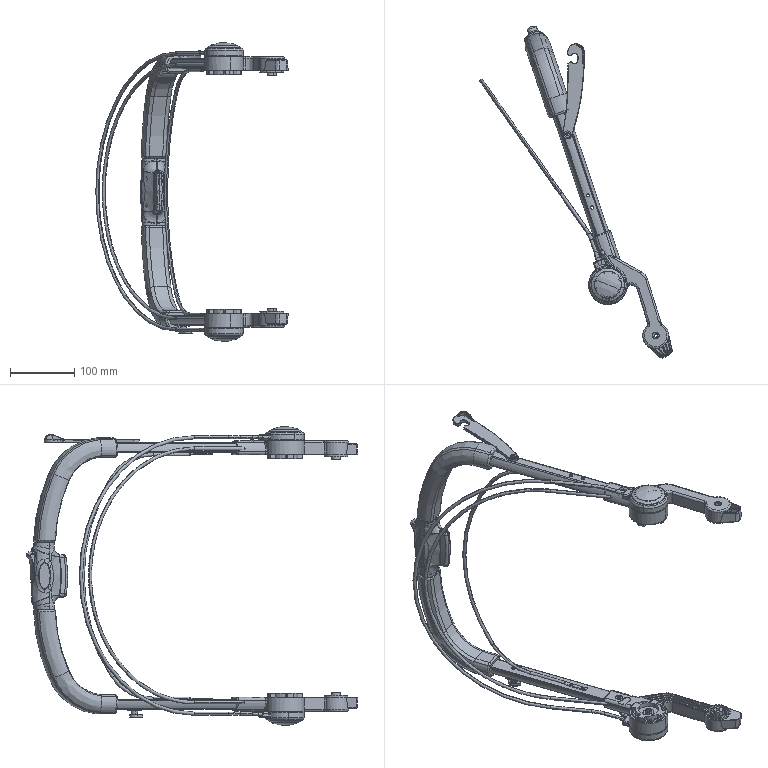Part | SolidWorks | 23 solids | 4172 faces | volume 744445 mm3 | spline 1534 | plane 1207 | cylinder 1169 | cone 118 | torus 98 | sphere 46 | commonest cylinder face diameters 1 x94 0.6 x65 2 x60 5.2 x50 4 x43 1.003 x40